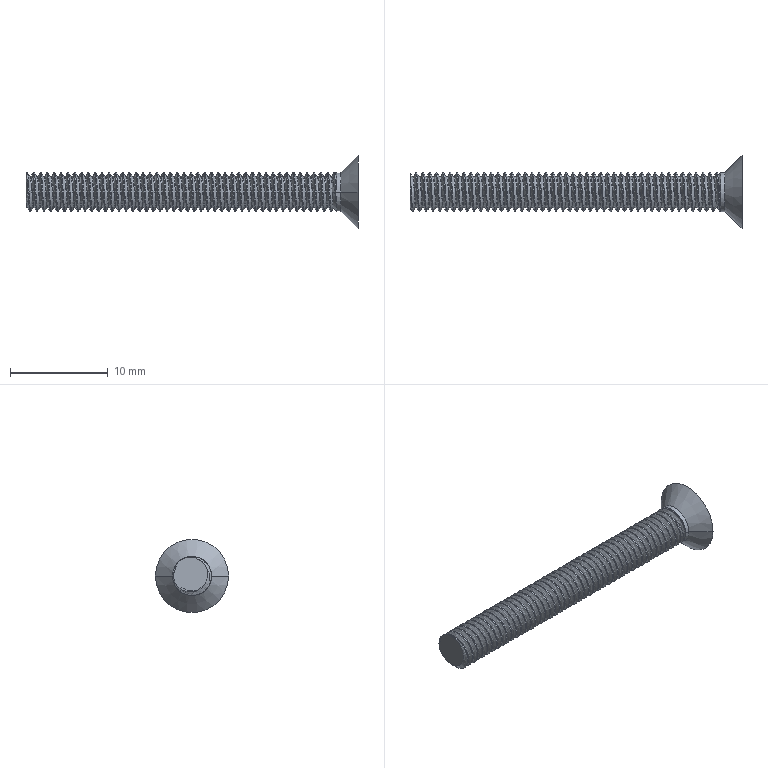Part | NX | features solid 2 | 1 solid | 212 faces | box 34 x 7.5 x 7.5 mm | volume 353.045 mm3 | cylinder 180 | plane 18 | cone 12 | spline 2 | commonest cylinder face diameters 4 x91 3.091 x89